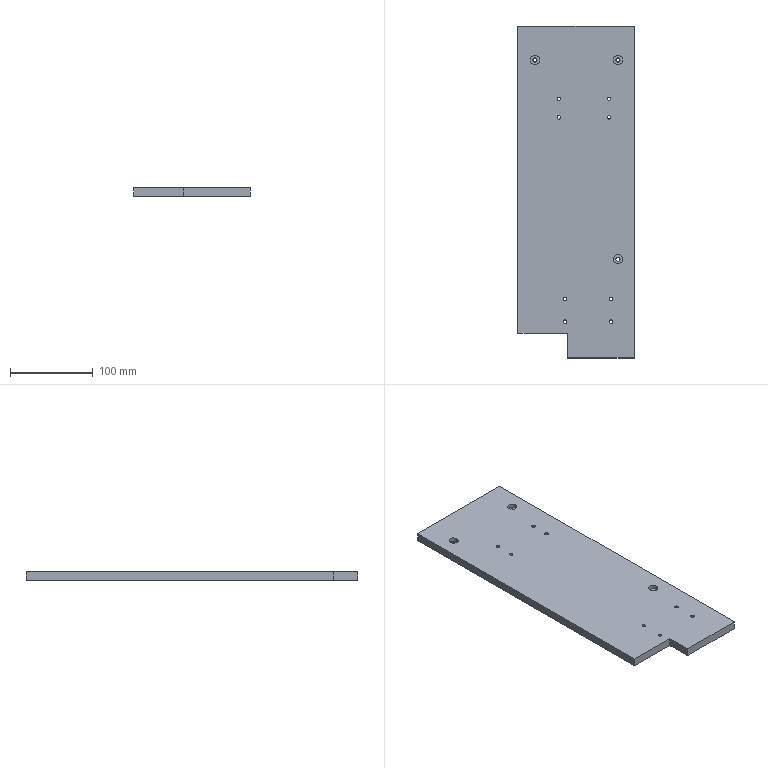Part | SolidWorks | features Cut 1, Extrusion 1, ICE 1 | 1 solid | 39 faces | box 140 x 400 x 10 mm | volume 539172 mm3 | cylinder 28 | plane 11 | commonest cylinder face diameters 4.2 x16 5 x6 11 x6
STEP:
#1=CARTESIAN_POINT('',(15.491,258.253,5.));
#2=VERTEX_POINT('',#1);
#3=CARTESIAN_POINT('',(26.491,258.253,5.));
#4=VERTEX_POINT('',#3);
#5=CARTESIAN_POINT('',(20.991,258.253,5.));
#6=DIRECTION('',(0.,0.,1.));
#7=DIRECTION('',(1.,0.,0.));
#8=AXIS2_PLACEMENT_3D('',#5,#6,#7);
#9=CIRCLE('',#8,5.5);
#10=EDGE_CURVE('',#2,#4,#9,.T.);
#11=ORIENTED_EDGE('',*,*,#10,.F.);
#12=CARTESIAN_POINT('',(15.491,258.253,10.));
#13=VERTEX_POINT('',#12);
#14=CARTESIAN_POINT('',(15.491,258.253,5.));
#15=DIRECTION('',(0.,0.,1.));
#16=VECTOR('',#15,1000.);
#17=LINE('',#14,#16);
#18=EDGE_CURVE('',#2,#13,#17,.T.);
#19=ORIENTED_EDGE('',*,*,#18,.T.);
#20=CARTESIAN_POINT('',(26.491,258.253,10.));
#21=VERTEX_POINT('',#20);
#22=CARTESIAN_POINT('',(20.991,258.253,10.));
#23=DIRECTION('',(0.,0.,1.));
#24=DIRECTION('',(1.,0.,0.));
#25=AXIS2_PLACEMENT_3D('',#22,#23,#24);
#26=CIRCLE('',#25,5.5);
#27=EDGE_CURVE('',#13,#21,#26,.T.);
#28=ORIENTED_EDGE('',*,*,#27,.T.);
#29=CARTESIAN_POINT('',(26.491,258.253,5.));
#30=DIRECTION('',(0.,0.,1.));
#31=VECTOR('',#30,1000.);
#32=LINE('',#29,#31);
#33=EDGE_CURVE('',#4,#21,#32,.T.);
#34=ORIENTED_EDGE('',*,*,#33,.F.);
#35=EDGE_LOOP('',(#11,#19,#28,#34));
#36=FACE_OUTER_BOUND('',#35,.T.);
#37=CARTESIAN_POINT('',(20.991,258.253,5.));
#38=DIRECTION('',(0.,0.,1.));
#39=DIRECTION('',(1.,0.,0.));
#40=AXIS2_PLACEMENT_3D('',#37,#38,#39);
#41=CYLINDRICAL_SURFACE('',#40,5.5);
#42=ADVANCED_FACE('',(#36),#41,.F.);
#43=CARTESIAN_POINT('',(15.491,18.253,5.));
#44=VERTEX_POINT('',#43);
#45=CARTESIAN_POINT('',(26.491,18.253,5.));
#46=VERTEX_POINT('',#45);
#47=CARTESIAN_POINT('',(20.991,18.253,5.));
#48=DIRECTION('',(0.,0.,1.));
#49=DIRECTION('',(1.,0.,0.));
#50=AXIS2_PLACEMENT_3D('',#47,#48,#49);
#51=CIRCLE('',#50,5.5);
#52=EDGE_CURVE('',#44,#46,#51,.T.);
#53=ORIENTED_EDGE('',*,*,#52,.F.);
#54=CARTESIAN_POINT('',(15.491,18.253,10.));
#55=VERTEX_POINT('',#54);
#56=CARTESIAN_POINT('',(15.491,18.253,5.));
#57=DIRECTION('',(0.,0.,1.));
#58=VECTOR('',#57,1000.);
#59=LINE('',#56,#58);
#60=EDGE_CURVE('',#44,#55,#59,.T.);
#61=ORIENTED_EDGE('',*,*,#60,.T.);
#62=CARTESIAN_POINT('',(26.491,18.253,10.));
#63=VERTEX_POINT('',#62);
#64=CARTESIAN_POINT('',(20.991,18.253,10.));
#65=DIRECTION('',(0.,0.,1.));
#66=DIRECTION('',(1.,0.,0.));
#67=AXIS2_PLACEMENT_3D('',#64,#65,#66);
#68=CIRCLE('',#67,5.5);
#69=EDGE_CURVE('',#55,#63,#68,.T.);
#70=ORIENTED_EDGE('',*,*,#69,.T.);
#71=CARTESIAN_POINT('',(26.491,18.253,5.));
#72=DIRECTION('',(0.,0.,1.));
#73=VECTOR('',#72,1000.);
#74=LINE('',#71,#73);
#75=EDGE_CURVE('',#46,#63,#74,.T.);
#76=ORIENTED_EDGE('',*,*,#75,.F.);
#77=EDGE_LOOP('',(#53,#61,#70,#76));
#78=FACE_OUTER_BOUND('',#77,.T.);
#79=CARTESIAN_POINT('',(20.991,18.253,5.));
#80=DIRECTION('',(0.,0.,1.));
#81=DIRECTION('',(1.,0.,0.));
#82=AXIS2_PLACEMENT_3D('',#79,#80,#81);
#83=CYLINDRICAL_SURFACE('',#82,5.5);
#84=ADVANCED_FACE('',(#78),#83,.F.);
#85=CARTESIAN_POINT('',(-84.509,258.294,5.));
#86=VERTEX_POINT('',#85);
#87=CARTESIAN_POINT('',(-73.509,258.294,5.));
#88=VERTEX_POINT('',#87);
#89=CARTESIAN_POINT('',(-79.009,258.294,5.));
#90=DIRECTION('',(0.,0.,1.));
#91=DIRECTION('',(1.,0.,0.));
#92=AXIS2_PLACEMENT_3D('',#89,#90,#91);
#93=CIRCLE('',#92,5.5);
#94=EDGE_CURVE('',#86,#88,#93,.T.);
#95=ORIENTED_EDGE('',*,*,#94,.F.);
#96=CARTESIAN_POINT('',(-84.509,258.294,10.));
#97=VERTEX_POINT('',#96);
#98=CARTESIAN_POINT('',(-84.509,258.294,5.));
#99=DIRECTION('',(0.,0.,1.));
#100=VECTOR('',#99,1000.);
#101=LINE('',#98,#100);
#102=EDGE_CURVE('',#86,#97,#101,.T.);
#103=ORIENTED_EDGE('',*,*,#102,.T.);
#104=CARTESIAN_POINT('',(-73.509,258.294,10.));
#105=VERTEX_POINT('',#104);
#106=CARTESIAN_POINT('',(-79.009,258.294,10.));
#107=DIRECTION('',(0.,0.,1.));
#108=DIRECTION('',(1.,0.,0.));
#109=AXIS2_PLACEMENT_3D('',#106,#107,#108);
#110=CIRCLE('',#109,5.5);
#111=EDGE_CURVE('',#97,#105,#110,.T.);
#112=ORIENTED_EDGE('',*,*,#111,.T.);
#113=CARTESIAN_POINT('',(-73.509,258.294,5.));
#114=DIRECTION('',(0.,0.,1.));
#115=VECTOR('',#114,1000.);
#116=LINE('',#113,#115);
#117=EDGE_CURVE('',#88,#105,#116,.T.);
#118=ORIENTED_EDGE('',*,*,#117,.F.);
#119=EDGE_LOOP('',(#95,#103,#112,#118));
#120=FACE_OUTER_BOUND('',#119,.T.);
#121=CARTESIAN_POINT('',(-79.009,258.294,5.));
#122=DIRECTION('',(0.,0.,1.));
#123=DIRECTION('',(1.,0.,0.));
#124=AXIS2_PLACEMENT_3D('',#121,#122,#123);
#125=CYLINDRICAL_SURFACE('',#124,5.5);
#126=ADVANCED_FACE('',(#120),#125,.F.);
#127=CARTESIAN_POINT('',(14.807,-29.519,0.));
#128=VERTEX_POINT('',#127);
#129=CARTESIAN_POINT('',(10.607,-29.519,0.));
#130=VERTEX_POINT('',#129);
#131=CARTESIAN_POINT('',(12.707,-29.519,0.));
#132=DIRECTION('',(0.,0.,-1.));
#133=DIRECTION('',(1.,0.,0.));
#134=AXIS2_PLACEMENT_3D('',#131,#132,#133);
#135=CIRCLE('',#134,2.1);
#136=EDGE_CURVE('',#128,#130,#135,.T.);
#137=ORIENTED_EDGE('',*,*,#136,.T.);
#138=CARTESIAN_POINT('',(10.607,-29.519,10.));
#139=VERTEX_POINT('',#138);
#140=CARTESIAN_POINT('',(10.607,-29.519,-7.071));
#141=DIRECTION('',(0.,0.,1.));
#142=VECTOR('',#141,1000.);
#143=LINE('',#140,#142);
#144=EDGE_CURVE('',#130,#139,#143,.T.);
#145=ORIENTED_EDGE('',*,*,#144,.T.);
#146=CARTESIAN_POINT('',(14.807,-29.519,10.));
#147=VERTEX_POINT('',#146);
#148=CARTESIAN_POINT('',(12.707,-29.519,10.));
#149=DIRECTION('',(0.,0.,1.));
#150=DIRECTION('',(1.,0.,0.));
#151=AXIS2_PLACEMENT_3D('',#148,#149,#150);
#152=CIRCLE('',#151,2.1);
#153=EDGE_CURVE('',#139,#147,#152,.T.);
#154=ORIENTED_EDGE('',*,*,#153,.T.);
#155=CARTESIAN_POINT('',(14.807,-29.519,-7.071));
#156=DIRECTION('',(0.,0.,1.));
#157=VECTOR('',#156,1000.);
#158=LINE('',#155,#157);
#159=EDGE_CURVE('',#128,#147,#158,.T.);
#160=ORIENTED_EDGE('',*,*,#159,.F.);
#161=EDGE_LOOP('',(#137,#145,#154,#160));
#162=FACE_OUTER_BOUND('',#161,.T.);
#163=CARTESIAN_POINT('',(12.707,-29.519,-7.071));
#164=DIRECTION('',(0.,0.,1.));
#165=DIRECTION('',(1.,0.,0.));
#166=AXIS2_PLACEMENT_3D('',#163,#164,#165);
#167=CYLINDRICAL_SURFACE('',#166,2.1);
#168=ADVANCED_FACE('',(#162),#167,.F.);
#169=CARTESIAN_POINT('',(12.27,211.583,0.));
#170=VERTEX_POINT('',#169);
#171=CARTESIAN_POINT('',(8.07,211.583,0.));
#172=VERTEX_POINT('',#171);
#173=CARTESIAN_POINT('',(10.17,211.583,0.));
#174=DIRECTION('',(0.,0.,-1.));
#175=DIRECTION('',(1.,0.,0.));
#176=AXIS2_PLACEMENT_3D('',#173,#174,#175);
#177=CIRCLE('',#176,2.1);
#178=EDGE_CURVE('',#170,#172,#177,.T.);
#179=ORIENTED_EDGE('',*,*,#178,.T.);
#180=CARTESIAN_POINT('',(8.07,211.583,10.));
#181=VERTEX_POINT('',#180);
#182=CARTESIAN_POINT('',(8.07,211.583,-7.071));
#183=DIRECTION('',(0.,0.,1.));
#184=VECTOR('',#183,1000.);
#185=LINE('',#182,#184);
#186=EDGE_CURVE('',#172,#181,#185,.T.);
#187=ORIENTED_EDGE('',*,*,#186,.T.);
#188=CARTESIAN_POINT('',(12.27,211.583,10.));
#189=VERTEX_POINT('',#188);
#190=CARTESIAN_POINT('',(10.17,211.583,10.));
#191=DIRECTION('',(0.,0.,1.));
#192=DIRECTION('',(1.,0.,0.));
#193=AXIS2_PLACEMENT_3D('',#190,#191,#192);
#194=CIRCLE('',#193,2.1);
#195=EDGE_CURVE('',#181,#189,#194,.T.);
#196=ORIENTED_EDGE('',*,*,#195,.T.);
#197=CARTESIAN_POINT('',(12.27,211.583,-7.071));
#198=DIRECTION('',(0.,0.,1.));
#199=VECTOR('',#198,1000.);
#200=LINE('',#197,#199);
#201=EDGE_CURVE('',#170,#189,#200,.T.);
#202=ORIENTED_EDGE('',*,*,#201,.F.);
#203=EDGE_LOOP('',(#179,#187,#196,#202));
#204=FACE_OUTER_BOUND('',#203,.T.);
#205=CARTESIAN_POINT('',(10.17,211.583,-7.071));
#206=DIRECTION('',(0.,0.,1.));
#207=DIRECTION('',(1.,0.,0.));
#208=AXIS2_PLACEMENT_3D('',#205,#206,#207);
#209=CYLINDRICAL_SURFACE('',#208,2.1);
#210=ADVANCED_FACE('',(#204),#209,.F.);
#211=CARTESIAN_POINT('',(-48.23,189.083,0.));
#212=VERTEX_POINT('',#211);
#213=CARTESIAN_POINT('',(-52.43,189.083,0.));
#214=VERTEX_POINT('',#213);
#215=CARTESIAN_POINT('',(-50.33,189.083,0.));
#216=DIRECTION('',(0.,0.,-1.));
#217=DIRECTION('',(1.,0.,0.));
#218=AXIS2_PLACEMENT_3D('',#215,#216,#217);
#219=CIRCLE('',#218,2.1);
#220=EDGE_CURVE('',#212,#214,#219,.T.);
#221=ORIENTED_EDGE('',*,*,#220,.T.);
#222=CARTESIAN_POINT('',(-52.43,189.083,10.));
#223=VERTEX_POINT('',#222);
#224=CARTESIAN_POINT('',(-52.43,189.083,-7.071));
#225=DIRECTION('',(0.,0.,1.));
#226=VECTOR('',#225,1000.);
#227=LINE('',#224,#226);
#228=EDGE_CURVE('',#214,#223,#227,.T.);
#229=ORIENTED_EDGE('',*,*,#228,.T.);
#230=CARTESIAN_POINT('',(-48.23,189.083,10.));
#231=VERTEX_POINT('',#230);
#232=CARTESIAN_POINT('',(-50.33,189.083,10.));
#233=DIRECTION('',(0.,0.,1.));
#234=DIRECTION('',(1.,0.,0.));
#235=AXIS2_PLACEMENT_3D('',#232,#233,#234);
#236=CIRCLE('',#235,2.1);
#237=EDGE_CURVE('',#223,#231,#236,.T.);
#238=ORIENTED_EDGE('',*,*,#237,.T.);
#239=CARTESIAN_POINT('',(-48.23,189.083,-7.071));
#240=DIRECTION('',(0.,0.,1.));
#241=VECTOR('',#240,1000.);
#242=LINE('',#239,#241);
#243=EDGE_CURVE('',#212,#231,#242,.T.);
#244=ORIENTED_EDGE('',*,*,#243,.F.);
#245=EDGE_LOOP('',(#221,#229,#238,#244));
#246=FACE_OUTER_BOUND('',#245,.T.);
#247=CARTESIAN_POINT('',(-50.33,189.083,-7.071));
#248=DIRECTION('',(0.,0.,1.));
#249=DIRECTION('',(1.,0.,0.));
#250=AXIS2_PLACEMENT_3D('',#247,#248,#249);
#251=CYLINDRICAL_SURFACE('',#250,2.1);
#252=ADVANCED_FACE('',(#246),#251,.F.);
#253=CARTESIAN_POINT('',(-48.23,211.583,0.));
#254=VERTEX_POINT('',#253);
#255=CARTESIAN_POINT('',(-52.43,211.583,0.));
#256=VERTEX_POINT('',#255);
#257=CARTESIAN_POINT('',(-50.33,211.583,0.));
#258=DIRECTION('',(0.,0.,-1.));
#259=DIRECTION('',(1.,0.,0.));
#260=AXIS2_PLACEMENT_3D('',#257,#258,#259);
#261=CIRCLE('',#260,2.1);
#262=EDGE_CURVE('',#254,#256,#261,.T.);
#263=ORIENTED_EDGE('',*,*,#262,.T.);
#264=CARTESIAN_POINT('',(-52.43,211.583,10.));
#265=VERTEX_POINT('',#264);
#266=CARTESIAN_POINT('',(-52.43,211.583,-7.071));
#267=DIRECTION('',(0.,0.,1.));
#268=VECTOR('',#267,1000.);
#269=LINE('',#266,#268);
#270=EDGE_CURVE('',#256,#265,#269,.T.);
#271=ORIENTED_EDGE('',*,*,#270,.T.);
#272=CARTESIAN_POINT('',(-48.23,211.583,10.));
#273=VERTEX_POINT('',#272);
#274=CARTESIAN_POINT('',(-50.33,211.583,10.));
#275=DIRECTION('',(0.,0.,1.));
#276=DIRECTION('',(1.,0.,0.));
#277=AXIS2_PLACEMENT_3D('',#274,#275,#276);
#278=CIRCLE('',#277,2.1);
#279=EDGE_CURVE('',#265,#273,#278,.T.);
#280=ORIENTED_EDGE('',*,*,#279,.T.);
#281=CARTESIAN_POINT('',(-48.23,211.583,-7.071));
#282=DIRECTION('',(0.,0.,1.));
#283=VECTOR('',#282,1000.);
#284=LINE('',#281,#283);
#285=EDGE_CURVE('',#254,#273,#284,.T.);
#286=ORIENTED_EDGE('',*,*,#285,.F.);
#287=EDGE_LOOP('',(#263,#271,#280,#286));
#288=FACE_OUTER_BOUND('',#287,.T.);
#289=CARTESIAN_POINT('',(-50.33,211.583,-7.071));
#290=DIRECTION('',(0.,0.,1.));
#291=DIRECTION('',(1.,0.,0.));
#292=AXIS2_PLACEMENT_3D('',#289,#290,#291);
#293=CYLINDRICAL_SURFACE('',#292,2.1);
#294=ADVANCED_FACE('',(#288),#293,.F.);
#295=CARTESIAN_POINT('',(12.27,189.083,0.));
#296=VERTEX_POINT('',#295);
#297=CARTESIAN_POINT('',(8.07,189.083,0.));
#298=VERTEX_POINT('',#297);
#299=CARTESIAN_POINT('',(10.17,189.083,0.));
#300=DIRECTION('',(0.,0.,-1.));
#301=DIRECTION('',(1.,0.,0.));
#302=AXIS2_PLACEMENT_3D('',#299,#300,#301);
#303=CIRCLE('',#302,2.1);
#304=EDGE_CURVE('',#296,#298,#303,.T.);
#305=ORIENTED_EDGE('',*,*,#304,.T.);
#306=CARTESIAN_POINT('',(8.07,189.083,10.));
#307=VERTEX_POINT('',#306);
#308=CARTESIAN_POINT('',(8.07,189.083,-7.071));
#309=DIRECTION('',(0.,0.,1.));
#310=VECTOR('',#309,1000.);
#311=LINE('',#308,#310);
#312=EDGE_CURVE('',#298,#307,#311,.T.);
#313=ORIENTED_EDGE('',*,*,#312,.T.);
#314=CARTESIAN_POINT('',(12.27,189.083,10.));
#315=VERTEX_POINT('',#314);
#316=CARTESIAN_POINT('',(10.17,189.083,10.));
#317=DIRECTION('',(0.,0.,1.));
#318=DIRECTION('',(1.,0.,0.));
#319=AXIS2_PLACEMENT_3D('',#316,#317,#318);
#320=CIRCLE('',#319,2.1);
#321=EDGE_CURVE('',#307,#315,#320,.T.);
#322=ORIENTED_EDGE('',*,*,#321,.T.);
#323=CARTESIAN_POINT('',(12.27,189.083,-7.071));
#324=DIRECTION('',(0.,0.,1.));
#325=VECTOR('',#324,1000.);
#326=LINE('',#323,#325);
#327=EDGE_CURVE('',#296,#315,#326,.T.);
#328=ORIENTED_EDGE('',*,*,#327,.F.);
#329=EDGE_LOOP('',(#305,#313,#322,#328));
#330=FACE_OUTER_BOUND('',#329,.T.);
#331=CARTESIAN_POINT('',(10.17,189.083,-7.071));
#332=DIRECTION('',(0.,0.,1.));
#333=DIRECTION('',(1.,0.,0.));
#334=AXIS2_PLACEMENT_3D('',#331,#332,#333);
#335=CYLINDRICAL_SURFACE('',#334,2.1);
#336=ADVANCED_FACE('',(#330),#335,.F.);
#337=CARTESIAN_POINT('',(-40.617,-29.519,0.));
#338=VERTEX_POINT('',#337);
#339=CARTESIAN_POINT('',(-44.817,-29.519,0.));
#340=VERTEX_POINT('',#339);
#341=CARTESIAN_POINT('',(-42.717,-29.519,0.));
#342=DIRECTION('',(0.,0.,-1.));
#343=DIRECTION('',(1.,0.,0.));
#344=AXIS2_PLACEMENT_3D('',#341,#342,#343);
#345=CIRCLE('',#344,2.1);
#346=EDGE_CURVE('',#338,#340,#345,.T.);
#347=ORIENTED_EDGE('',*,*,#346,.T.);
#348=CARTESIAN_POINT('',(-44.817,-29.519,10.));
#349=VERTEX_POINT('',#348);
#350=CARTESIAN_POINT('',(-44.817,-29.519,-7.071));
#351=DIRECTION('',(0.,0.,1.));
#352=VECTOR('',#351,1000.);
#353=LINE('',#350,#352);
#354=EDGE_CURVE('',#340,#349,#353,.T.);
#355=ORIENTED_EDGE('',*,*,#354,.T.);
#356=CARTESIAN_POINT('',(-40.617,-29.519,10.));
#357=VERTEX_POINT('',#356);
#358=CARTESIAN_POINT('',(-42.717,-29.519,10.));
#359=DIRECTION('',(0.,0.,1.));
#360=DIRECTION('',(1.,0.,0.));
#361=AXIS2_PLACEMENT_3D('',#358,#359,#360);
#362=CIRCLE('',#361,2.1);
#363=EDGE_CURVE('',#349,#357,#362,.T.);
#364=ORIENTED_EDGE('',*,*,#363,.T.);
#365=CARTESIAN_POINT('',(-40.617,-29.519,-7.071));
#366=DIRECTION('',(0.,0.,1.));
#367=VECTOR('',#366,1000.);
#368=LINE('',#365,#367);
#369=EDGE_CURVE('',#338,#357,#368,.T.);
#370=ORIENTED_EDGE('',*,*,#369,.F.);
#371=EDGE_LOOP('',(#347,#355,#364,#370));
#372=FACE_OUTER_BOUND('',#371,.T.);
#373=CARTESIAN_POINT('',(-42.717,-29.519,-7.071));
#374=DIRECTION('',(0.,0.,1.));
#375=DIRECTION('',(1.,0.,0.));
#376=AXIS2_PLACEMENT_3D('',#373,#374,#375);
#377=CYLINDRICAL_SURFACE('',#376,2.1);
#378=ADVANCED_FACE('',(#372),#377,.F.);
#379=CARTESIAN_POINT('',(-40.617,-57.019,0.));
#380=VERTEX_POINT('',#379);
#381=CARTESIAN_POINT('',(-44.817,-57.019,0.));
#382=VERTEX_POINT('',#381);
#383=CARTESIAN_POINT('',(-42.717,-57.019,0.));
#384=DIRECTION('',(0.,0.,-1.));
#385=DIRECTION('',(1.,0.,0.));
#386=AXIS2_PLACEMENT_3D('',#383,#384,#385);
#387=CIRCLE('',#386,2.1);
#388=EDGE_CURVE('',#380,#382,#387,.T.);
#389=ORIENTED_EDGE('',*,*,#388,.T.);
#390=CARTESIAN_POINT('',(-44.817,-57.019,10.));
#391=VERTEX_POINT('',#390);
#392=CARTESIAN_POINT('',(-44.817,-57.019,-7.071));
#393=DIRECTION('',(0.,0.,1.));
#394=VECTOR('',#393,1000.);
#395=LINE('',#392,#394);
#396=EDGE_CURVE('',#382,#391,#395,.T.);
#397=ORIENTED_EDGE('',*,*,#396,.T.);
#398=CARTESIAN_POINT('',(-40.617,-57.019,10.));
#399=VERTEX_POINT('',#398);
#400=CARTESIAN_POINT('',(-42.717,-57.019,10.));
#401=DIRECTION('',(0.,0.,1.));
#402=DIRECTION('',(1.,0.,0.));
#403=AXIS2_PLACEMENT_3D('',#400,#401,#402);
#404=CIRCLE('',#403,2.1);
#405=EDGE_CURVE('',#391,#399,#404,.T.);
#406=ORIENTED_EDGE('',*,*,#405,.T.);
#407=CARTESIAN_POINT('',(-40.617,-57.019,-7.071));
#408=DIRECTION('',(0.,0.,1.));
#409=VECTOR('',#408,1000.);
#410=LINE('',#407,#409);
#411=EDGE_CURVE('',#380,#399,#410,.T.);
#412=ORIENTED_EDGE('',*,*,#411,.F.);
#413=EDGE_LOOP('',(#389,#397,#406,#412));
#414=FACE_OUTER_BOUND('',#413,.T.);
#415=CARTESIAN_POINT('',(-42.717,-57.019,-7.071));
#416=DIRECTION('',(0.,0.,1.));
#417=DIRECTION('',(1.,0.,0.));
#418=AXIS2_PLACEMENT_3D('',#415,#416,#417);
#419=CYLINDRICAL_SURFACE('',#418,2.1);
#420=ADVANCED_FACE('',(#414),#419,.F.);
#421=CARTESIAN_POINT('',(14.807,-57.019,0.));
#422=VERTEX_POINT('',#421);
#423=CARTESIAN_POINT('',(10.607,-57.019,0.));
#424=VERTEX_POINT('',#423);
#425=CARTESIAN_POINT('',(12.707,-57.019,0.));
#426=DIRECTION('',(0.,0.,-1.));
#427=DIRECTION('',(1.,0.,0.));
#428=AXIS2_PLACEMENT_3D('',#425,#426,#427);
#429=CIRCLE('',#428,2.1);
#430=EDGE_CURVE('',#422,#424,#429,.T.);
#431=ORIENTED_EDGE('',*,*,#430,.T.);
#432=CARTESIAN_POINT('',(10.607,-57.019,10.));
#433=VERTEX_POINT('',#432);
#434=CARTESIAN_POINT('',(10.607,-57.019,-7.071));
#435=DIRECTION('',(0.,0.,1.));
#436=VECTOR('',#435,1000.);
#437=LINE('',#434,#436);
#438=EDGE_CURVE('',#424,#433,#437,.T.);
#439=ORIENTED_EDGE('',*,*,#438,.T.);
#440=CARTESIAN_POINT('',(14.807,-57.019,10.));
#441=VERTEX_POINT('',#440);
#442=CARTESIAN_POINT('',(12.707,-57.019,10.));
#443=DIRECTION('',(0.,0.,1.));
#444=DIRECTION('',(1.,0.,0.));
#445=AXIS2_PLACEMENT_3D('',#442,#443,#444);
#446=CIRCLE('',#445,2.1);
#447=EDGE_CURVE('',#433,#441,#446,.T.);
#448=ORIENTED_EDGE('',*,*,#447,.T.);
#449=CARTESIAN_POINT('',(14.807,-57.019,-7.071));
#450=DIRECTION('',(0.,0.,1.));
#451=VECTOR('',#450,1000.);
#452=LINE('',#449,#451);
#453=EDGE_CURVE('',#422,#441,#452,.T.);
#454=ORIENTED_EDGE('',*,*,#453,.F.);
#455=EDGE_LOOP('',(#431,#439,#448,#454));
#456=FACE_OUTER_BOUND('',#455,.T.);
#457=CARTESIAN_POINT('',(12.707,-57.019,-7.071));
#458=DIRECTION('',(0.,0.,1.));
#459=DIRECTION('',(1.,0.,0.));
#460=AXIS2_PLACEMENT_3D('',#457,#458,#459);
#461=CYLINDRICAL_SURFACE('',#460,2.1);
#462=ADVANCED_FACE('',(#456),#461,.F.);
#463=CARTESIAN_POINT('',(-76.509,258.253,0.));
#464=VERTEX_POINT('',#463);
#465=CARTESIAN_POINT('',(-81.509,258.253,0.));
#466=VERTEX_POINT('',#465);
#467=CARTESIAN_POINT('',(-79.009,258.253,0.));
#468=DIRECTION('',(0.,0.,-1.));
#469=DIRECTION('',(1.,0.,0.));
#470=AXIS2_PLACEMENT_3D('',#467,#468,#469);
#471=CIRCLE('',#470,2.5);
#472=EDGE_CURVE('',#464,#466,#471,.T.);
#473=ORIENTED_EDGE('',*,*,#472,.T.);
#474=CARTESIAN_POINT('',(-81.509,258.253,5.));
#475=VERTEX_POINT('',#474);
#476=CARTESIAN_POINT('',(-81.509,258.253,-7.071));
#477=DIRECTION('',(0.,0.,1.));
#478=VECTOR('',#477,1000.);
#479=LINE('',#476,#478);
#480=EDGE_CURVE('',#466,#475,#479,.T.);
#481=ORIENTED_EDGE('',*,*,#480,.T.);
#482=CARTESIAN_POINT('',(-76.509,258.253,5.));
#483=VERTEX_POINT('',#482);
#484=CARTESIAN_POINT('',(-79.009,258.253,5.));
#485=DIRECTION('',(0.,0.,-1.));
#486=DIRECTION('',(1.,0.,0.));
#487=AXIS2_PLACEMENT_3D('',#484,#485,#486);
#488=CIRCLE('',#487,2.5);
#489=EDGE_CURVE('',#483,#475,#488,.T.);
#490=ORIENTED_EDGE('',*,*,#489,.F.);
#491=CARTESIAN_POINT('',(-76.509,258.253,-7.071));
#492=DIRECTION('',(0.,0.,1.));
#493=VECTOR('',#492,1000.);
#494=LINE('',#491,#493);
#495=EDGE_CURVE('',#464,#483,#494,.T.);
#496=ORIENTED_EDGE('',*,*,#495,.F.);
#497=EDGE_LOOP('',(#473,#481,#490,#496));
#498=FACE_OUTER_BOUND('',#497,.T.);
#499=CARTESIAN_POINT('',(-79.009,258.253,-7.071));
#500=DIRECTION('',(0.,0.,1.));
#501=DIRECTION('',(1.,0.,0.));
#502=AXIS2_PLACEMENT_3D('',#499,#500,#501);
#503=CYLINDRICAL_SURFACE('',#502,2.5);
#504=ADVANCED_FACE('',(#498),#503,.F.);
#505=CARTESIAN_POINT('',(23.491,18.253,0.));
#506=VERTEX_POINT('',#505);
#507=CARTESIAN_POINT('',(18.491,18.253,0.));
#508=VERTEX_POINT('',#507);
#509=CARTESIAN_POINT('',(20.991,18.253,0.));
#510=DIRECTION('',(0.,0.,-1.));
#511=DIRECTION('',(1.,0.,0.));
#512=AXIS2_PLACEMENT_3D('',#509,#510,#511);
#513=CIRCLE('',#512,2.5);
#514=EDGE_CURVE('',#506,#508,#513,.T.);
#515=ORIENTED_EDGE('',*,*,#514,.T.);
#516=CARTESIAN_POINT('',(18.491,18.253,5.));
#517=VERTEX_POINT('',#516);
#518=CARTESIAN_POINT('',(18.491,18.253,-7.071));
#519=DIRECTION('',(0.,0.,1.));
#520=VECTOR('',#519,1000.);
#521=LINE('',#518,#520);
#522=EDGE_CURVE('',#508,#517,#521,.T.);
#523=ORIENTED_EDGE('',*,*,#522,.T.);
#524=CARTESIAN_POINT('',(23.491,18.253,5.));
#525=VERTEX_POINT('',#524);
#526=CARTESIAN_POINT('',(20.991,18.253,5.));
#527=DIRECTION('',(0.,0.,-1.));
#528=DIRECTION('',(1.,0.,0.));
#529=AXIS2_PLACEMENT_3D('',#526,#527,#528);
#530=CIRCLE('',#529,2.5);
#531=EDGE_CURVE('',#525,#517,#530,.T.);
#532=ORIENTED_EDGE('',*,*,#531,.F.);
#533=CARTESIAN_POINT('',(23.491,18.253,-7.071));
#534=DIRECTION('',(0.,0.,1.));
#535=VECTOR('',#534,1000.);
#536=LINE('',#533,#535);
#537=EDGE_CURVE('',#506,#525,#536,.T.);
#538=ORIENTED_EDGE('',*,*,#537,.F.);
#539=EDGE_LOOP('',(#515,#523,#532,#538));
#540=FACE_OUTER_BOUND('',#539,.T.);
#541=CARTESIAN_POINT('',(20.991,18.253,-7.071));
#542=DIRECTION('',(0.,0.,1.));
#543=DIRECTION('',(1.,0.,0.));
#544=AXIS2_PLACEMENT_3D('',#541,#542,#543);
#545=CYLINDRICAL_SURFACE('',#544,2.5);
#546=ADVANCED_FACE('',(#540),#545,.F.);
#547=CARTESIAN_POINT('',(23.491,258.253,0.));
#548=VERTEX_POINT('',#547);
#549=CARTESIAN_POINT('',(18.491,258.253,0.));
#550=VERTEX_POINT('',#549);
#551=CARTESIAN_POINT('',(20.991,258.253,0.));
#552=DIRECTION('',(0.,0.,-1.));
#553=DIRECTION('',(1.,0.,0.));
#554=AXIS2_PLACEMENT_3D('',#551,#552,#553);
#555=CIRCLE('',#554,2.5);
#556=EDGE_CURVE('',#548,#550,#555,.T.);
#557=ORIENTED_EDGE('',*,*,#556,.T.);
#558=CARTESIAN_POINT('',(18.491,258.253,5.));
#559=VERTEX_POINT('',#558);
#560=CARTESIAN_POINT('',(18.491,258.253,-7.071));
#561=DIRECTION('',(0.,0.,1.));
#562=VECTOR('',#561,1000.);
#563=LINE('',#560,#562);
#564=EDGE_CURVE('',#550,#559,#563,.T.);
#565=ORIENTED_EDGE('',*,*,#564,.T.);
#566=CARTESIAN_POINT('',(23.491,258.253,5.));
#567=VERTEX_POINT('',#566);
#568=CARTESIAN_POINT('',(20.991,258.253,5.));
#569=DIRECTION('',(0.,0.,-1.));
#570=DIRECTION('',(1.,0.,0.));
#571=AXIS2_PLACEMENT_3D('',#568,#569,#570);
#572=CIRCLE('',#571,2.5);
#573=EDGE_CURVE('',#567,#559,#572,.T.);
#574=ORIENTED_EDGE('',*,*,#573,.F.);
#575=CARTESIAN_POINT('',(23.491,258.253,-7.071));
#576=DIRECTION('',(0.,0.,1.));
#577=VECTOR('',#576,1000.);
#578=LINE('',#575,#577);
#579=EDGE_CURVE('',#548,#567,#578,.T.);
#580=ORIENTED_EDGE('',*,*,#579,.F.);
#581=EDGE_LOOP('',(#557,#565,#574,#580));
#582=FACE_OUTER_BOUND('',#581,.T.);
#583=CARTESIAN_POINT('',(20.991,258.253,-7.071));
#584=DIRECTION('',(0.,0.,1.));
#585=DIRECTION('',(1.,0.,0.));
#586=AXIS2_PLACEMENT_3D('',#583,#584,#585);
#587=CYLINDRICAL_SURFACE('',#586,2.5);
#588=ADVANCED_FACE('',(#582),#587,.F.);
#589=ORIENTED_EDGE('',*,*,#564,.F.);
#590=CARTESIAN_POINT('',(20.991,258.253,0.));
#591=DIRECTION('',(0.,0.,-1.));
#592=DIRECTION('',(1.,0.,0.));
#593=AXIS2_PLACEMENT_3D('',#590,#591,#592);
#594=CIRCLE('',#593,2.5);
#595=EDGE_CURVE('',#550,#548,#594,.T.);
#596=ORIENTED_EDGE('',*,*,#595,.T.);
#597=ORIENTED_EDGE('',*,*,#579,.T.);
#598=CARTESIAN_POINT('',(20.991,258.253,5.));
#599=DIRECTION('',(0.,0.,-1.));
#600=DIRECTION('',(1.,0.,0.));
#601=AXIS2_PLACEMENT_3D('',#598,#599,#600);
#602=CIRCLE('',#601,2.5);
#603=EDGE_CURVE('',#559,#567,#602,.T.);
#604=ORIENTED_EDGE('',*,*,#603,.F.);
#605=EDGE_LOOP('',(#589,#596,#597,#604));
#606=FACE_OUTER_BOUND('',#605,.T.);
#607=CARTESIAN_POINT('',(20.991,258.253,-7.071));
#608=DIRECTION('',(0.,0.,1.));
#609=DIRECTION('',(1.,0.,0.));
#610=AXIS2_PLACEMENT_3D('',#607,#608,#609);
#611=CYLINDRICAL_SURFACE('',#610,2.5);
#612=ADVANCED_FACE('',(#606),#611,.F.);
#613=ORIENTED_EDGE('',*,*,#522,.F.);
#614=CARTESIAN_POINT('',(20.991,18.253,0.));
#615=DIRECTION('',(0.,0.,-1.));
#616=DIRECTION('',(1.,0.,0.));
#617=AXIS2_PLACEMENT_3D('',#614,#615,#616);
#618=CIRCLE('',#617,2.5);
#619=EDGE_CURVE('',#508,#506,#618,.T.);
#620=ORIENTED_EDGE('',*,*,#619,.T.);
#621=ORIENTED_EDGE('',*,*,#537,.T.);
#622=CARTESIAN_POINT('',(20.991,18.253,5.));
#623=DIRECTION('',(0.,0.,-1.));
#624=DIRECTION('',(1.,0.,0.));
#625=AXIS2_PLACEMENT_3D('',#622,#623,#624);
#626=CIRCLE('',#625,2.5);
#627=EDGE_CURVE('',#517,#525,#626,.T.);
#628=ORIENTED_EDGE('',*,*,#627,.F.);
#629=EDGE_LOOP('',(#613,#620,#621,#628));
#630=FACE_OUTER_BOUND('',#629,.T.);
#631=CARTESIAN_POINT('',(20.991,18.253,-7.071));
#632=DIRECTION('',(0.,0.,1.));
#633=DIRECTION('',(1.,0.,0.));
#634=AXIS2_PLACEMENT_3D('',#631,#632,#633);
#635=CYLINDRICAL_SURFACE('',#634,2.5);
#636=ADVANCED_FACE('',(#630),#635,.F.);
#637=ORIENTED_EDGE('',*,*,#480,.F.);
#638=CARTESIAN_POINT('',(-79.009,258.253,0.));
#639=DIRECTION('',(0.,0.,-1.));
#640=DIRECTION('',(1.,0.,0.));
#641=AXIS2_PLACEMENT_3D('',#638,#639,#640);
#642=CIRCLE('',#641,2.5);
#643=EDGE_CURVE('',#466,#464,#642,.T.);
#644=ORIENTED_EDGE('',*,*,#643,.T.);
#645=ORIENTED_EDGE('',*,*,#495,.T.);
#646=CARTESIAN_POINT('',(-79.009,258.253,5.));
#647=DIRECTION('',(0.,0.,-1.));
#648=DIRECTION('',(1.,0.,0.));
#649=AXIS2_PLACEMENT_3D('',#646,#647,#648);
#650=CIRCLE('',#649,2.5);
#651=EDGE_CURVE('',#475,#483,#650,.T.);
#652=ORIENTED_EDGE('',*,*,#651,.F.);
#653=EDGE_LOOP('',(#637,#644,#645,#652));
#654=FACE_OUTER_BOUND('',#653,.T.);
#655=CARTESIAN_POINT('',(-79.009,258.253,-7.071));
#656=DIRECTION('',(0.,0.,1.));
#657=DIRECTION('',(1.,0.,0.));
#658=AXIS2_PLACEMENT_3D('',#655,#656,#657);
#659=CYLINDRICAL_SURFACE('',#658,2.5);
#660=ADVANCED_FACE('',(#654),#659,.F.);
#661=CARTESIAN_POINT('',(-99.58,299.231,0.));
#662=VERTEX_POINT('',#661);
#663=CARTESIAN_POINT('',(-99.58,-70.769,0.));
#664=VERTEX_POINT('',#663);
#665=CARTESIAN_POINT('',(-99.58,299.231,0.));
#666=DIRECTION('',(0.,-1.,0.));
#667=VECTOR('',#666,1000.);
#668=LINE('',#665,#667);
#669=EDGE_CURVE('',#662,#664,#668,.T.);
#670=ORIENTED_EDGE('',*,*,#669,.T.);
#671=CARTESIAN_POINT('',(-99.58,-70.769,10.));
#672=VERTEX_POINT('',#671);
#673=CARTESIAN_POINT('',(-99.58,-70.769,10.));
#674=DIRECTION('',(0.,0.,-1.));
#675=VECTOR('',#674,1000.);
#676=LINE('',#673,#675);
#677=EDGE_CURVE('',#672,#664,#676,.T.);
#678=ORIENTED_EDGE('',*,*,#677,.F.);
#679=CARTESIAN_POINT('',(-99.58,299.231,10.));
#680=VERTEX_POINT('',#679);
#681=CARTESIAN_POINT('',(-99.58,299.231,10.));
#682=DIRECTION('',(0.,-1.,0.));
#683=VECTOR('',#682,1000.);
#684=LINE('',#681,#683);
#685=EDGE_CURVE('',#680,#672,#684,.T.);
#686=ORIENTED_EDGE('',*,*,#685,.F.);
#687=CARTESIAN_POINT('',(-99.58,299.231,10.));
#688=DIRECTION('',(0.,0.,-1.));
#689=VECTOR('',#688,1000.);
#690=LINE('',#687,#689);
#691=EDGE_CURVE('',#680,#662,#690,.T.);
#692=ORIENTED_EDGE('',*,*,#691,.T.);
#693=EDGE_LOOP('',(#670,#678,#686,#692));
#694=FACE_OUTER_BOUND('',#693,.T.);
#695=CARTESIAN_POINT('',(-99.58,299.231,10.));
#696=DIRECTION('',(1.,0.,0.));
#697=DIRECTION('',(0.,1.,0.));
#698=AXIS2_PLACEMENT_3D('',#695,#696,#697);
#699=PLANE('',#698);
#700=ADVANCED_FACE('',(#694),#699,.F.);
#701=CARTESIAN_POINT('',(-39.58,-70.769,0.));
#702=VERTEX_POINT('',#701);
#703=CARTESIAN_POINT('',(-99.58,-70.769,0.));
#704=DIRECTION('',(1.,0.,0.));
#705=VECTOR('',#704,1000.);
#706=LINE('',#703,#705);
#707=EDGE_CURVE('',#664,#702,#706,.T.);
#708=ORIENTED_EDGE('',*,*,#707,.T.);
#709=CARTESIAN_POINT('',(-39.58,-70.769,10.));
#710=VERTEX_POINT('',#709);
#711=CARTESIAN_POINT('',(-39.58,-70.769,10.));
#712=DIRECTION('',(0.,0.,-1.));
#713=VECTOR('',#712,1000.);
#714=LINE('',#711,#713);
#715=EDGE_CURVE('',#710,#702,#714,.T.);
#716=ORIENTED_EDGE('',*,*,#715,.F.);
#717=CARTESIAN_POINT('',(-99.58,-70.769,10.));
#718=DIRECTION('',(1.,0.,0.));
#719=VECTOR('',#718,1000.);
#720=LINE('',#717,#719);
#721=EDGE_CURVE('',#672,#710,#720,.T.);
#722=ORIENTED_EDGE('',*,*,#721,.F.);
#723=ORIENTED_EDGE('',*,*,#677,.T.);
#724=EDGE_LOOP('',(#708,#716,#722,#723));
#725=FACE_OUTER_BOUND('',#724,.T.);
#726=CARTESIAN_POINT('',(-99.58,-70.769,10.));
#727=DIRECTION('',(0.,1.,0.));
#728=DIRECTION('',(0.,0.,1.));
#729=AXIS2_PLACEMENT_3D('',#726,#727,#728);
#730=PLANE('',#729);
#731=ADVANCED_FACE('',(#725),#730,.F.);
#732=CARTESIAN_POINT('',(-39.58,-100.769,0.));
#733=VERTEX_POINT('',#732);
#734=CARTESIAN_POINT('',(-39.58,-70.769,0.));
#735=DIRECTION('',(0.,-1.,0.));
#736=VECTOR('',#735,1000.);
#737=LINE('',#734,#736);
#738=EDGE_CURVE('',#702,#733,#737,.T.);
#739=ORIENTED_EDGE('',*,*,#738,.T.);
#740=CARTESIAN_POINT('',(-39.58,-100.769,10.));
#741=VERTEX_POINT('',#740);
#742=CARTESIAN_POINT('',(-39.58,-100.769,10.));
#743=DIRECTION('',(0.,0.,-1.));
#744=VECTOR('',#743,1000.);
#745=LINE('',#742,#744);
#746=EDGE_CURVE('',#741,#733,#745,.T.);
#747=ORIENTED_EDGE('',*,*,#746,.F.);
#748=CARTESIAN_POINT('',(-39.58,-70.769,10.));
#749=DIRECTION('',(0.,-1.,0.));
#750=VECTOR('',#749,1000.);
#751=LINE('',#748,#750);
#752=EDGE_CURVE('',#710,#741,#751,.T.);
#753=ORIENTED_EDGE('',*,*,#752,.F.);
#754=ORIENTED_EDGE('',*,*,#715,.T.);
#755=EDGE_LOOP('',(#739,#747,#753,#754));
#756=FACE_OUTER_BOUND('',#755,.T.);
#757=CARTESIAN_POINT('',(-39.58,-70.769,10.));
#758=DIRECTION('',(1.,0.,0.));
#759=DIRECTION('',(0.,0.,-1.));
#760=AXIS2_PLACEMENT_3D('',#757,#758,#759);
#761=PLANE('',#760);
#762=ADVANCED_FACE('',(#756),#761,.F.);
#763=CARTESIAN_POINT('',(40.42,-100.769,0.));
#764=VERTEX_POINT('',#763);
#765=CARTESIAN_POINT('',(-39.58,-100.769,0.));
#766=DIRECTION('',(1.,0.,0.));
#767=VECTOR('',#766,1000.);
#768=LINE('',#765,#767);
#769=EDGE_CURVE('',#733,#764,#768,.T.);
#770=ORIENTED_EDGE('',*,*,#769,.T.);
#771=CARTESIAN_POINT('',(40.42,-100.769,10.));
#772=VERTEX_POINT('',#771);
#773=CARTESIAN_POINT('',(40.42,-100.769,10.));
#774=DIRECTION('',(0.,0.,-1.));
#775=VECTOR('',#774,1000.);
#776=LINE('',#773,#775);
#777=EDGE_CURVE('',#772,#764,#776,.T.);
#778=ORIENTED_EDGE('',*,*,#777,.F.);
#779=CARTESIAN_POINT('',(-39.58,-100.769,10.));
#780=DIRECTION('',(1.,0.,0.));
#781=VECTOR('',#780,1000.);
#782=LINE('',#779,#781);
#783=EDGE_CURVE('',#741,#772,#782,.T.);
#784=ORIENTED_EDGE('',*,*,#783,.F.);
#785=ORIENTED_EDGE('',*,*,#746,.T.);
#786=EDGE_LOOP('',(#770,#778,#784,#785));
#787=FACE_OUTER_BOUND('',#786,.T.);
#788=CARTESIAN_POINT('',(-39.58,-100.769,10.));
#789=DIRECTION('',(0.,1.,0.));
#790=DIRECTION('',(0.,0.,1.));
#791=AXIS2_PLACEMENT_3D('',#788,#789,#790);
#792=PLANE('',#791);
#793=ADVANCED_FACE('',(#787),#792,.F.);
#794=CARTESIAN_POINT('',(40.42,299.231,0.));
#795=VERTEX_POINT('',#794);
#796=CARTESIAN_POINT('',(40.42,-100.769,0.));
#797=DIRECTION('',(0.,1.,0.));
#798=VECTOR('',#797,1000.);
#799=LINE('',#796,#798);
#800=EDGE_CURVE('',#764,#795,#799,.T.);
#801=ORIENTED_EDGE('',*,*,#800,.T.);
#802=CARTESIAN_POINT('',(40.42,299.231,10.));
#803=VERTEX_POINT('',#802);
#804=CARTESIAN_POINT('',(40.42,299.231,10.));
#805=DIRECTION('',(0.,0.,-1.));
#806=VECTOR('',#805,1000.);
#807=LINE('',#804,#806);
#808=EDGE_CURVE('',#803,#795,#807,.T.);
#809=ORIENTED_EDGE('',*,*,#808,.F.);
#810=CARTESIAN_POINT('',(40.42,-100.769,10.));
#811=DIRECTION('',(0.,1.,0.));
#812=VECTOR('',#811,1000.);
#813=LINE('',#810,#812);
#814=EDGE_CURVE('',#772,#803,#813,.T.);
#815=ORIENTED_EDGE('',*,*,#814,.F.);
#816=ORIENTED_EDGE('',*,*,#777,.T.);
#817=EDGE_LOOP('',(#801,#809,#815,#816));
#818=FACE_OUTER_BOUND('',#817,.T.);
#819=CARTESIAN_POINT('',(40.42,-100.769,10.));
#820=DIRECTION('',(-1.,0.,0.));
#821=DIRECTION('',(0.,0.,1.));
#822=AXIS2_PLACEMENT_3D('',#819,#820,#821);
#823=PLANE('',#822);
#824=ADVANCED_FACE('',(#818),#823,.F.);
#825=CARTESIAN_POINT('',(40.42,299.231,0.));
#826=DIRECTION('',(-1.,0.,0.));
#827=VECTOR('',#826,1000.);
#828=LINE('',#825,#827);
#829=EDGE_CURVE('',#795,#662,#828,.T.);
#830=ORIENTED_EDGE('',*,*,#829,.T.);
#831=ORIENTED_EDGE('',*,*,#691,.F.);
#832=CARTESIAN_POINT('',(40.42,299.231,10.));
#833=DIRECTION('',(-1.,0.,0.));
#834=VECTOR('',#833,1000.);
#835=LINE('',#832,#834);
#836=EDGE_CURVE('',#803,#680,#835,.T.);
#837=ORIENTED_EDGE('',*,*,#836,.F.);
#838=ORIENTED_EDGE('',*,*,#808,.T.);
#839=EDGE_LOOP('',(#830,#831,#837,#838));
#840=FACE_OUTER_BOUND('',#839,.T.);
#841=CARTESIAN_POINT('',(40.42,299.231,10.));
#842=DIRECTION('',(0.,-1.,0.));
#843=DIRECTION('',(0.,0.,-1.));
#844=AXIS2_PLACEMENT_3D('',#841,#842,#843);
#845=PLANE('',#844);
#846=ADVANCED_FACE('',(#840),#845,.F.);
#847=CARTESIAN_POINT('',(20.991,18.253,10.));
#848=DIRECTION('',(0.,0.,1.));
#849=DIRECTION('',(1.,0.,0.));
#850=AXIS2_PLACEMENT_3D('',#847,#848,#849);
#851=CIRCLE('',#850,5.5);
#852=EDGE_CURVE('',#63,#55,#851,.T.);
#853=ORIENTED_EDGE('',*,*,#852,.F.);
#854=ORIENTED_EDGE('',*,*,#69,.F.);
#855=EDGE_LOOP('',(#853,#854));
#856=FACE_BOUND('',#855,.T.);
#857=CARTESIAN_POINT('',(-79.009,258.294,10.));
#858=DIRECTION('',(0.,0.,1.));
#859=DIRECTION('',(1.,0.,0.));
#860=AXIS2_PLACEMENT_3D('',#857,#858,#859);
#861=CIRCLE('',#860,5.5);
#862=EDGE_CURVE('',#105,#97,#861,.T.);
#863=ORIENTED_EDGE('',*,*,#862,.F.);
#864=ORIENTED_EDGE('',*,*,#111,.F.);
#865=EDGE_LOOP('',(#863,#864));
#866=FACE_BOUND('',#865,.T.);
#867=CARTESIAN_POINT('',(20.991,258.253,10.));
#868=DIRECTION('',(0.,0.,1.));
#869=DIRECTION('',(1.,0.,0.));
#870=AXIS2_PLACEMENT_3D('',#867,#868,#869);
#871=CIRCLE('',#870,5.5);
#872=EDGE_CURVE('',#21,#13,#871,.T.);
#873=ORIENTED_EDGE('',*,*,#872,.F.);
#874=ORIENTED_EDGE('',*,*,#27,.F.);
#875=EDGE_LOOP('',(#873,#874));
#876=FACE_BOUND('',#875,.T.);
#877=CARTESIAN_POINT('',(12.707,-29.519,10.));
#878=DIRECTION('',(0.,0.,1.));
#879=DIRECTION('',(1.,0.,0.));
#880=AXIS2_PLACEMENT_3D('',#877,#878,#879);
#881=CIRCLE('',#880,2.1);
#882=EDGE_CURVE('',#147,#139,#881,.T.);
#883=ORIENTED_EDGE('',*,*,#882,.F.);
#884=ORIENTED_EDGE('',*,*,#153,.F.);
#885=EDGE_LOOP('',(#883,#884));
#886=FACE_BOUND('',#885,.T.);
#887=CARTESIAN_POINT('',(10.17,211.583,10.));
#888=DIRECTION('',(0.,0.,1.));
#889=DIRECTION('',(1.,0.,0.));
#890=AXIS2_PLACEMENT_3D('',#887,#888,#889);
#891=CIRCLE('',#890,2.1);
#892=EDGE_CURVE('',#189,#181,#891,.T.);
#893=ORIENTED_EDGE('',*,*,#892,.F.);
#894=ORIENTED_EDGE('',*,*,#195,.F.);
#895=EDGE_LOOP('',(#893,#894));
#896=FACE_BOUND('',#895,.T.);
#897=CARTESIAN_POINT('',(-50.33,189.083,10.));
#898=DIRECTION('',(0.,0.,1.));
#899=DIRECTION('',(1.,0.,0.));
#900=AXIS2_PLACEMENT_3D('',#897,#898,#899);
#901=CIRCLE('',#900,2.1);
#902=EDGE_CURVE('',#231,#223,#901,.T.);
#903=ORIENTED_EDGE('',*,*,#902,.F.);
#904=ORIENTED_EDGE('',*,*,#237,.F.);
#905=EDGE_LOOP('',(#903,#904));
#906=FACE_BOUND('',#905,.T.);
#907=CARTESIAN_POINT('',(-50.33,211.583,10.));
#908=DIRECTION('',(0.,0.,1.));
#909=DIRECTION('',(1.,0.,0.));
#910=AXIS2_PLACEMENT_3D('',#907,#908,#909);
#911=CIRCLE('',#910,2.1);
#912=EDGE_CURVE('',#273,#265,#911,.T.);
#913=ORIENTED_EDGE('',*,*,#912,.F.);
#914=ORIENTED_EDGE('',*,*,#279,.F.);
#915=EDGE_LOOP('',(#913,#914));
#916=FACE_BOUND('',#915,.T.);
#917=CARTESIAN_POINT('',(10.17,189.083,10.));
#918=DIRECTION('',(0.,0.,1.));
#919=DIRECTION('',(1.,0.,0.));
#920=AXIS2_PLACEMENT_3D('',#917,#918,#919);
#921=CIRCLE('',#920,2.1);
#922=EDGE_CURVE('',#315,#307,#921,.T.);
#923=ORIENTED_EDGE('',*,*,#922,.F.);
#924=ORIENTED_EDGE('',*,*,#321,.F.);
#925=EDGE_LOOP('',(#923,#924));
#926=FACE_BOUND('',#925,.T.);
#927=CARTESIAN_POINT('',(-42.717,-29.519,10.));
#928=DIRECTION('',(0.,0.,1.));
#929=DIRECTION('',(1.,0.,0.));
#930=AXIS2_PLACEMENT_3D('',#927,#928,#929);
#931=CIRCLE('',#930,2.1);
#932=EDGE_CURVE('',#357,#349,#931,.T.);
#933=ORIENTED_EDGE('',*,*,#932,.F.);
#934=ORIENTED_EDGE('',*,*,#363,.F.);
#935=EDGE_LOOP('',(#933,#934));
#936=FACE_BOUND('',#935,.T.);
#937=CARTESIAN_POINT('',(-42.717,-57.019,10.));
#938=DIRECTION('',(0.,0.,1.));
#939=DIRECTION('',(1.,0.,0.));
#940=AXIS2_PLACEMENT_3D('',#937,#938,#939);
#941=CIRCLE('',#940,2.1);
#942=EDGE_CURVE('',#399,#391,#941,.T.);
#943=ORIENTED_EDGE('',*,*,#942,.F.);
#944=ORIENTED_EDGE('',*,*,#405,.F.);
#945=EDGE_LOOP('',(#943,#944));
#946=FACE_BOUND('',#945,.T.);
#947=CARTESIAN_POINT('',(12.707,-57.019,10.));
#948=DIRECTION('',(0.,0.,1.));
#949=DIRECTION('',(1.,0.,0.));
#950=AXIS2_PLACEMENT_3D('',#947,#948,#949);
#951=CIRCLE('',#950,2.1);
#952=EDGE_CURVE('',#441,#433,#951,.T.);
#953=ORIENTED_EDGE('',*,*,#952,.F.);
#954=ORIENTED_EDGE('',*,*,#447,.F.);
#955=EDGE_LOOP('',(#953,#954));
#956=FACE_BOUND('',#955,.T.);
#957=ORIENTED_EDGE('',*,*,#685,.T.);
#958=ORIENTED_EDGE('',*,*,#721,.T.);
#959=ORIENTED_EDGE('',*,*,#752,.T.);
#960=ORIENTED_EDGE('',*,*,#783,.T.);
#961=ORIENTED_EDGE('',*,*,#814,.T.);
#962=ORIENTED_EDGE('',*,*,#836,.T.);
#963=EDGE_LOOP('',(#957,#958,#959,#960,#961,#962));
#964=FACE_OUTER_BOUND('',#963,.T.);
#965=CARTESIAN_POINT('',(0.,0.,10.));
#966=DIRECTION('',(0.,0.,1.));
#967=DIRECTION('',(1.,0.,0.));
#968=AXIS2_PLACEMENT_3D('',#965,#966,#967);
#969=PLANE('',#968);
#970=ADVANCED_FACE('',(#856,#866,#876,#886,#896,#906,#916,#926,#936,#946,#956,#964),#969,.T.);
#971=ORIENTED_EDGE('',*,*,#472,.F.);
#972=ORIENTED_EDGE('',*,*,#643,.F.);
#973=EDGE_LOOP('',(#971,#972));
#974=FACE_BOUND('',#973,.T.);
#975=ORIENTED_EDGE('',*,*,#514,.F.);
#976=ORIENTED_EDGE('',*,*,#619,.F.);
#977=EDGE_LOOP('',(#975,#976));
#978=FACE_BOUND('',#977,.T.);
#979=ORIENTED_EDGE('',*,*,#136,.F.);
#980=CARTESIAN_POINT('',(12.707,-29.519,0.));
#981=DIRECTION('',(0.,0.,-1.));
#982=DIRECTION('',(1.,0.,0.));
#983=AXIS2_PLACEMENT_3D('',#980,#981,#982);
#984=CIRCLE('',#983,2.1);
#985=EDGE_CURVE('',#130,#128,#984,.T.);
#986=ORIENTED_EDGE('',*,*,#985,.F.);
#987=EDGE_LOOP('',(#979,#986));
#988=FACE_BOUND('',#987,.T.);
#989=ORIENTED_EDGE('',*,*,#178,.F.);
#990=CARTESIAN_POINT('',(10.17,211.583,0.));
#991=DIRECTION('',(0.,0.,-1.));
#992=DIRECTION('',(1.,0.,0.));
#993=AXIS2_PLACEMENT_3D('',#990,#991,#992);
#994=CIRCLE('',#993,2.1);
#995=EDGE_CURVE('',#172,#170,#994,.T.);
#996=ORIENTED_EDGE('',*,*,#995,.F.);
#997=EDGE_LOOP('',(#989,#996));
#998=FACE_BOUND('',#997,.T.);
#999=ORIENTED_EDGE('',*,*,#220,.F.);
#1000=CARTESIAN_POINT('',(-50.33,189.083,0.));
#1001=DIRECTION('',(0.,0.,-1.));
#1002=DIRECTION('',(1.,0.,0.));
#1003=AXIS2_PLACEMENT_3D('',#1000,#1001,#1002);
#1004=CIRCLE('',#1003,2.1);
#1005=EDGE_CURVE('',#214,#212,#1004,.T.);
#1006=ORIENTED_EDGE('',*,*,#1005,.F.);
#1007=EDGE_LOOP('',(#999,#1006));
#1008=FACE_BOUND('',#1007,.T.);
#1009=ORIENTED_EDGE('',*,*,#262,.F.);
#1010=CARTESIAN_POINT('',(-50.33,211.583,0.));
#1011=DIRECTION('',(0.,0.,-1.));
#1012=DIRECTION('',(1.,0.,0.));
#1013=AXIS2_PLACEMENT_3D('',#1010,#1011,#1012);
#1014=CIRCLE('',#1013,2.1);
#1015=EDGE_CURVE('',#256,#254,#1014,.T.);
#1016=ORIENTED_EDGE('',*,*,#1015,.F.);
#1017=EDGE_LOOP('',(#1009,#1016));
#1018=FACE_BOUND('',#1017,.T.);
#1019=ORIENTED_EDGE('',*,*,#556,.F.);
#1020=ORIENTED_EDGE('',*,*,#595,.F.);
#1021=EDGE_LOOP('',(#1019,#1020));
#1022=FACE_BOUND('',#1021,.T.);
#1023=ORIENTED_EDGE('',*,*,#304,.F.);
#1024=CARTESIAN_POINT('',(10.17,189.083,0.));
#1025=DIRECTION('',(0.,0.,-1.));
#1026=DIRECTION('',(1.,0.,0.));
#1027=AXIS2_PLACEMENT_3D('',#1024,#1025,#1026);
#1028=CIRCLE('',#1027,2.1);
#1029=EDGE_CURVE('',#298,#296,#1028,.T.);
#1030=ORIENTED_EDGE('',*,*,#1029,.F.);
#1031=EDGE_LOOP('',(#1023,#1030));
#1032=FACE_BOUND('',#1031,.T.);
#1033=ORIENTED_EDGE('',*,*,#346,.F.);
#1034=CARTESIAN_POINT('',(-42.717,-29.519,0.));
#1035=DIRECTION('',(0.,0.,-1.));
#1036=DIRECTION('',(1.,0.,0.));
#1037=AXIS2_PLACEMENT_3D('',#1034,#1035,#1036);
#1038=CIRCLE('',#1037,2.1);
#1039=EDGE_CURVE('',#340,#338,#1038,.T.);
#1040=ORIENTED_EDGE('',*,*,#1039,.F.);
#1041=EDGE_LOOP('',(#1033,#1040));
#1042=FACE_BOUND('',#1041,.T.);
#1043=ORIENTED_EDGE('',*,*,#388,.F.);
#1044=CARTESIAN_POINT('',(-42.717,-57.019,0.));
#1045=DIRECTION('',(0.,0.,-1.));
#1046=DIRECTION('',(1.,0.,0.));
#1047=AXIS2_PLACEMENT_3D('',#1044,#1045,#1046);
#1048=CIRCLE('',#1047,2.1);
#1049=EDGE_CURVE('',#382,#380,#1048,.T.);
#1050=ORIENTED_EDGE('',*,*,#1049,.F.);
#1051=EDGE_LOOP('',(#1043,#1050));
#1052=FACE_BOUND('',#1051,.T.);
#1053=ORIENTED_EDGE('',*,*,#430,.F.);
#1054=CARTESIAN_POINT('',(12.707,-57.019,0.));
#1055=DIRECTION('',(0.,0.,-1.));
#1056=DIRECTION('',(1.,0.,0.));
#1057=AXIS2_PLACEMENT_3D('',#1054,#1055,#1056);
#1058=CIRCLE('',#1057,2.1);
#1059=EDGE_CURVE('',#424,#422,#1058,.T.);
#1060=ORIENTED_EDGE('',*,*,#1059,.F.);
#1061=EDGE_LOOP('',(#1053,#1060));
#1062=FACE_BOUND('',#1061,.T.);
#1063=ORIENTED_EDGE('',*,*,#669,.F.);
#1064=ORIENTED_EDGE('',*,*,#829,.F.);
#1065=ORIENTED_EDGE('',*,*,#800,.F.);
#1066=ORIENTED_EDGE('',*,*,#769,.F.);
#1067=ORIENTED_EDGE('',*,*,#738,.F.);
#1068=ORIENTED_EDGE('',*,*,#707,.F.);
#1069=EDGE_LOOP('',(#1063,#1064,#1065,#1066,#1067,#1068));
#1070=FACE_OUTER_BOUND('',#1069,.T.);
#1071=CARTESIAN_POINT('',(0.,0.,0.));
#1072=DIRECTION('',(0.,0.,1.));
#1073=DIRECTION('',(1.,0.,0.));
#1074=AXIS2_PLACEMENT_3D('',#1071,#1072,#1073);
#1075=PLANE('',#1074);
#1076=ADVANCED_FACE('',(#974,#978,#988,#998,#1008,#1018,#1022,#1032,#1042,#1052,#1062,#1070),#1075,.F.);
#1077=ORIENTED_EDGE('',*,*,#438,.F.);
#1078=ORIENTED_EDGE('',*,*,#1059,.T.);
#1079=ORIENTED_EDGE('',*,*,#453,.T.);
#1080=ORIENTED_EDGE('',*,*,#952,.T.);
#1081=EDGE_LOOP('',(#1077,#1078,#1079,#1080));
#1082=FACE_OUTER_BOUND('',#1081,.T.);
#1083=CARTESIAN_POINT('',(12.707,-57.019,-7.071));
#1084=DIRECTION('',(0.,0.,1.));
#1085=DIRECTION('',(1.,0.,0.));
#1086=AXIS2_PLACEMENT_3D('',#1083,#1084,#1085);
#1087=CYLINDRICAL_SURFACE('',#1086,2.1);
#1088=ADVANCED_FACE('',(#1082),#1087,.F.);
#1089=ORIENTED_EDGE('',*,*,#396,.F.);
#1090=ORIENTED_EDGE('',*,*,#1049,.T.);
#1091=ORIENTED_EDGE('',*,*,#411,.T.);
#1092=ORIENTED_EDGE('',*,*,#942,.T.);
#1093=EDGE_LOOP('',(#1089,#1090,#1091,#1092));
#1094=FACE_OUTER_BOUND('',#1093,.T.);
#1095=CARTESIAN_POINT('',(-42.717,-57.019,-7.071));
#1096=DIRECTION('',(0.,0.,1.));
#1097=DIRECTION('',(1.,0.,0.));
#1098=AXIS2_PLACEMENT_3D('',#1095,#1096,#1097);
#1099=CYLINDRICAL_SURFACE('',#1098,2.1);
#1100=ADVANCED_FACE('',(#1094),#1099,.F.);
#1101=ORIENTED_EDGE('',*,*,#354,.F.);
#1102=ORIENTED_EDGE('',*,*,#1039,.T.);
#1103=ORIENTED_EDGE('',*,*,#369,.T.);
#1104=ORIENTED_EDGE('',*,*,#932,.T.);
#1105=EDGE_LOOP('',(#1101,#1102,#1103,#1104));
#1106=FACE_OUTER_BOUND('',#1105,.T.);
#1107=CARTESIAN_POINT('',(-42.717,-29.519,-7.071));
#1108=DIRECTION('',(0.,0.,1.));
#1109=DIRECTION('',(1.,0.,0.));
#1110=AXIS2_PLACEMENT_3D('',#1107,#1108,#1109);
#1111=CYLINDRICAL_SURFACE('',#1110,2.1);
#1112=ADVANCED_FACE('',(#1106),#1111,.F.);
#1113=ORIENTED_EDGE('',*,*,#312,.F.);
#1114=ORIENTED_EDGE('',*,*,#1029,.T.);
#1115=ORIENTED_EDGE('',*,*,#327,.T.);
#1116=ORIENTED_EDGE('',*,*,#922,.T.);
#1117=EDGE_LOOP('',(#1113,#1114,#1115,#1116));
#1118=FACE_OUTER_BOUND('',#1117,.T.);
#1119=CARTESIAN_POINT('',(10.17,189.083,-7.071));
#1120=DIRECTION('',(0.,0.,1.));
#1121=DIRECTION('',(1.,0.,0.));
#1122=AXIS2_PLACEMENT_3D('',#1119,#1120,#1121);
#1123=CYLINDRICAL_SURFACE('',#1122,2.1);
#1124=ADVANCED_FACE('',(#1118),#1123,.F.);
#1125=ORIENTED_EDGE('',*,*,#270,.F.);
#1126=ORIENTED_EDGE('',*,*,#1015,.T.);
#1127=ORIENTED_EDGE('',*,*,#285,.T.);
#1128=ORIENTED_EDGE('',*,*,#912,.T.);
#1129=EDGE_LOOP('',(#1125,#1126,#1127,#1128));
#1130=FACE_OUTER_BOUND('',#1129,.T.);
#1131=CARTESIAN_POINT('',(-50.33,211.583,-7.071));
#1132=DIRECTION('',(0.,0.,1.));
#1133=DIRECTION('',(1.,0.,0.));
#1134=AXIS2_PLACEMENT_3D('',#1131,#1132,#1133);
#1135=CYLINDRICAL_SURFACE('',#1134,2.1);
#1136=ADVANCED_FACE('',(#1130),#1135,.F.);
#1137=ORIENTED_EDGE('',*,*,#228,.F.);
#1138=ORIENTED_EDGE('',*,*,#1005,.T.);
#1139=ORIENTED_EDGE('',*,*,#243,.T.);
#1140=ORIENTED_EDGE('',*,*,#902,.T.);
#1141=EDGE_LOOP('',(#1137,#1138,#1139,#1140));
#1142=FACE_OUTER_BOUND('',#1141,.T.);
#1143=CARTESIAN_POINT('',(-50.33,189.083,-7.071));
#1144=DIRECTION('',(0.,0.,1.));
#1145=DIRECTION('',(1.,0.,0.));
#1146=AXIS2_PLACEMENT_3D('',#1143,#1144,#1145);
#1147=CYLINDRICAL_SURFACE('',#1146,2.1);
#1148=ADVANCED_FACE('',(#1142),#1147,.F.);
#1149=ORIENTED_EDGE('',*,*,#186,.F.);
#1150=ORIENTED_EDGE('',*,*,#995,.T.);
#1151=ORIENTED_EDGE('',*,*,#201,.T.);
#1152=ORIENTED_EDGE('',*,*,#892,.T.);
#1153=EDGE_LOOP('',(#1149,#1150,#1151,#1152));
#1154=FACE_OUTER_BOUND('',#1153,.T.);
#1155=CARTESIAN_POINT('',(10.17,211.583,-7.071));
#1156=DIRECTION('',(0.,0.,1.));
#1157=DIRECTION('',(1.,0.,0.));
#1158=AXIS2_PLACEMENT_3D('',#1155,#1156,#1157);
#1159=CYLINDRICAL_SURFACE('',#1158,2.1);
#1160=ADVANCED_FACE('',(#1154),#1159,.F.);
#1161=ORIENTED_EDGE('',*,*,#144,.F.);
#1162=ORIENTED_EDGE('',*,*,#985,.T.);
#1163=ORIENTED_EDGE('',*,*,#159,.T.);
#1164=ORIENTED_EDGE('',*,*,#882,.T.);
#1165=EDGE_LOOP('',(#1161,#1162,#1163,#1164));
#1166=FACE_OUTER_BOUND('',#1165,.T.);
#1167=CARTESIAN_POINT('',(12.707,-29.519,-7.071));
#1168=DIRECTION('',(0.,0.,1.));
#1169=DIRECTION('',(1.,0.,0.));
#1170=AXIS2_PLACEMENT_3D('',#1167,#1168,#1169);
#1171=CYLINDRICAL_SURFACE('',#1170,2.1);
#1172=ADVANCED_FACE('',(#1166),#1171,.F.);
#1173=CARTESIAN_POINT('',(-79.009,258.294,5.));
#1174=DIRECTION('',(0.,0.,1.));
#1175=DIRECTION('',(1.,0.,0.));
#1176=AXIS2_PLACEMENT_3D('',#1173,#1174,#1175);
#1177=CIRCLE('',#1176,5.5);
#1178=EDGE_CURVE('',#88,#86,#1177,.T.);
#1179=ORIENTED_EDGE('',*,*,#1178,.T.);
#1180=ORIENTED_EDGE('',*,*,#94,.T.);
#1181=EDGE_LOOP('',(#1179,#1180));
#1182=FACE_OUTER_BOUND('',#1181,.T.);
#1183=ORIENTED_EDGE('',*,*,#489,.T.);
#1184=ORIENTED_EDGE('',*,*,#651,.T.);
#1185=EDGE_LOOP('',(#1183,#1184));
#1186=FACE_BOUND('',#1185,.T.);
#1187=CARTESIAN_POINT('',(-79.009,258.294,5.));
#1188=DIRECTION('',(0.,0.,1.));
#1189=DIRECTION('',(1.,0.,0.));
#1190=AXIS2_PLACEMENT_3D('',#1187,#1188,#1189);
#1191=PLANE('',#1190);
#1192=ADVANCED_FACE('',(#1182,#1186),#1191,.T.);
#1193=ORIENTED_EDGE('',*,*,#102,.F.);
#1194=ORIENTED_EDGE('',*,*,#1178,.F.);
#1195=ORIENTED_EDGE('',*,*,#117,.T.);
#1196=ORIENTED_EDGE('',*,*,#862,.T.);
#1197=EDGE_LOOP('',(#1193,#1194,#1195,#1196));
#1198=FACE_OUTER_BOUND('',#1197,.T.);
#1199=CARTESIAN_POINT('',(-79.009,258.294,5.));
#1200=DIRECTION('',(0.,0.,1.));
#1201=DIRECTION('',(1.,0.,0.));
#1202=AXIS2_PLACEMENT_3D('',#1199,#1200,#1201);
#1203=CYLINDRICAL_SURFACE('',#1202,5.5);
#1204=ADVANCED_FACE('',(#1198),#1203,.F.);
#1205=CARTESIAN_POINT('',(20.991,18.253,5.));
#1206=DIRECTION('',(0.,0.,1.));
#1207=DIRECTION('',(1.,0.,0.));
#1208=AXIS2_PLACEMENT_3D('',#1205,#1206,#1207);
#1209=CIRCLE('',#1208,5.5);
#1210=EDGE_CURVE('',#46,#44,#1209,.T.);
#1211=ORIENTED_EDGE('',*,*,#1210,.T.);
#1212=ORIENTED_EDGE('',*,*,#52,.T.);
#1213=EDGE_LOOP('',(#1211,#1212));
#1214=FACE_OUTER_BOUND('',#1213,.T.);
#1215=ORIENTED_EDGE('',*,*,#531,.T.);
#1216=ORIENTED_EDGE('',*,*,#627,.T.);
#1217=EDGE_LOOP('',(#1215,#1216));
#1218=FACE_BOUND('',#1217,.T.);
#1219=CARTESIAN_POINT('',(20.991,18.253,5.));
#1220=DIRECTION('',(0.,0.,1.));
#1221=DIRECTION('',(1.,0.,0.));
#1222=AXIS2_PLACEMENT_3D('',#1219,#1220,#1221);
#1223=PLANE('',#1222);
#1224=ADVANCED_FACE('',(#1214,#1218),#1223,.T.);
#1225=ORIENTED_EDGE('',*,*,#60,.F.);
#1226=ORIENTED_EDGE('',*,*,#1210,.F.);
#1227=ORIENTED_EDGE('',*,*,#75,.T.);
#1228=ORIENTED_EDGE('',*,*,#852,.T.);
#1229=EDGE_LOOP('',(#1225,#1226,#1227,#1228));
#1230=FACE_OUTER_BOUND('',#1229,.T.);
#1231=CARTESIAN_POINT('',(20.991,18.253,5.));
#1232=DIRECTION('',(0.,0.,1.));
#1233=DIRECTION('',(1.,0.,0.));
#1234=AXIS2_PLACEMENT_3D('',#1231,#1232,#1233);
#1235=CYLINDRICAL_SURFACE('',#1234,5.5);
#1236=ADVANCED_FACE('',(#1230),#1235,.F.);
#1237=CARTESIAN_POINT('',(20.991,258.253,5.));
#1238=DIRECTION('',(0.,0.,1.));
#1239=DIRECTION('',(1.,0.,0.));
#1240=AXIS2_PLACEMENT_3D('',#1237,#1238,#1239);
#1241=CIRCLE('',#1240,5.5);
#1242=EDGE_CURVE('',#4,#2,#1241,.T.);
#1243=ORIENTED_EDGE('',*,*,#1242,.T.);
#1244=ORIENTED_EDGE('',*,*,#10,.T.);
#1245=EDGE_LOOP('',(#1243,#1244));
#1246=FACE_OUTER_BOUND('',#1245,.T.);
#1247=ORIENTED_EDGE('',*,*,#573,.T.);
#1248=ORIENTED_EDGE('',*,*,#603,.T.);
#1249=EDGE_LOOP('',(#1247,#1248));
#1250=FACE_BOUND('',#1249,.T.);
#1251=CARTESIAN_POINT('',(20.991,258.253,5.));
#1252=DIRECTION('',(0.,0.,1.));
#1253=DIRECTION('',(1.,0.,0.));
#1254=AXIS2_PLACEMENT_3D('',#1251,#1252,#1253);
#1255=PLANE('',#1254);
#1256=ADVANCED_FACE('',(#1246,#1250),#1255,.T.);
#1257=ORIENTED_EDGE('',*,*,#18,.F.);
#1258=ORIENTED_EDGE('',*,*,#1242,.F.);
#1259=ORIENTED_EDGE('',*,*,#33,.T.);
#1260=ORIENTED_EDGE('',*,*,#872,.T.);
#1261=EDGE_LOOP('',(#1257,#1258,#1259,#1260));
#1262=FACE_OUTER_BOUND('',#1261,.T.);
#1263=CARTESIAN_POINT('',(20.991,258.253,5.));
#1264=DIRECTION('',(0.,0.,1.));
#1265=DIRECTION('',(1.,0.,0.));
#1266=AXIS2_PLACEMENT_3D('',#1263,#1264,#1265);
#1267=CYLINDRICAL_SURFACE('',#1266,5.5);
#1268=ADVANCED_FACE('',(#1262),#1267,.F.);
#1269=CLOSED_SHELL('',(#42,#84,#126,#168,#210,#252,#294,#336,#378,#420,#462,#504,#546,#588,#612,#636,#660,#700,#731,#762,#793,#824,#846,#970,#1076,#1088,#1100,#1112,#1124,#1136,#1148,#1160,#1172,#1192,#1204,#1224,#1236,#1256,#1268));
#1270=MANIFOLD_SOLID_BREP('',#1269);
#1271=CARTESIAN_POINT('',(0.,0.,0.));
#1272=DIRECTION('',(0.,0.,1.));
#1273=DIRECTION('',(1.,0.,0.));
#1274=AXIS2_PLACEMENT_3D('',#1271,#1272,#1273);
#1275=(LENGTH_UNIT()NAMED_UNIT(*)SI_UNIT(.MILLI.,.METRE.));
#1276=UNCERTAINTY_MEASURE_WITH_UNIT(LENGTH_MEASURE(0.00001),#1275,'','');
#1277=(NAMED_UNIT(*)PLANE_ANGLE_UNIT()SI_UNIT($,.RADIAN.));
#1278=(NAMED_UNIT(*)SI_UNIT($,.STERADIAN.)SOLID_ANGLE_UNIT());
#1279=(GEOMETRIC_REPRESENTATION_CONTEXT(3)GLOBAL_UNCERTAINTY_ASSIGNED_CONTEXT((#1276))GLOBAL_UNIT_ASSIGNED_CONTEXT((#1275,#1277,#1278))REPRESENTATION_CONTEXT('',''));
#1280=ADVANCED_BREP_SHAPE_REPRESENTATION('',(#1270,#1274),#1279);